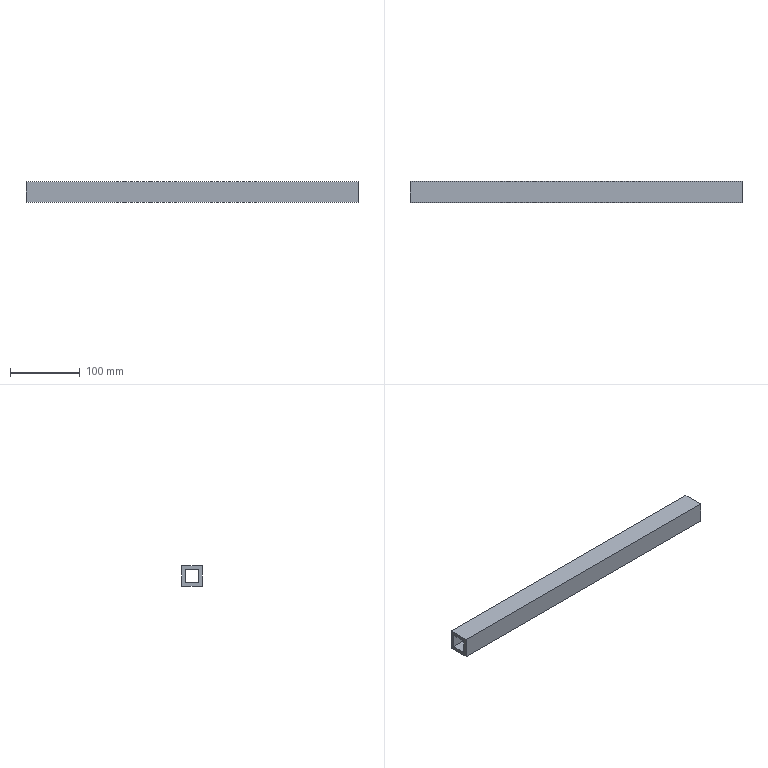Part | NX | features solid 2 | 1 solid | 10 faces | box 475 x 30 x 30 mm | volume 237500 mm3 | plane 10
STEP:
#1=CARTESIAN_POINT('',(650.,-165.,-80.));
#2=VERTEX_POINT('',#1);
#3=CARTESIAN_POINT('',(650.,-195.,-80.));
#4=VERTEX_POINT('',#3);
#5=CARTESIAN_POINT('',(650.,-165.,-80.));
#6=DIRECTION('',(0.,-1.,0.));
#7=VECTOR('',#6,1000.);
#8=LINE('',#5,#7);
#9=EDGE_CURVE('',#2,#4,#8,.T.);
#10=ORIENTED_EDGE('',*,*,#9,.F.);
#11=CARTESIAN_POINT('',(650.,-165.,-50.));
#12=VERTEX_POINT('',#11);
#13=CARTESIAN_POINT('',(650.,-165.,-50.));
#14=DIRECTION('',(0.,0.,-1.));
#15=VECTOR('',#14,1000.);
#16=LINE('',#13,#15);
#17=EDGE_CURVE('',#12,#2,#16,.T.);
#18=ORIENTED_EDGE('',*,*,#17,.F.);
#19=CARTESIAN_POINT('',(650.,-195.,-50.));
#20=VERTEX_POINT('',#19);
#21=CARTESIAN_POINT('',(650.,-165.,-50.));
#22=DIRECTION('',(0.,1.,0.));
#23=VECTOR('',#22,1000.);
#24=LINE('',#21,#23);
#25=EDGE_CURVE('',#12,#20,#24,.F.);
#26=ORIENTED_EDGE('',*,*,#25,.T.);
#27=CARTESIAN_POINT('',(650.,-195.,-50.));
#28=DIRECTION('',(0.,0.,1.));
#29=VECTOR('',#28,1000.);
#30=LINE('',#27,#29);
#31=EDGE_CURVE('',#20,#4,#30,.F.);
#32=ORIENTED_EDGE('',*,*,#31,.T.);
#33=EDGE_LOOP('',(#10,#18,#26,#32));
#34=FACE_BOUND('',#33,.T.);
#35=CARTESIAN_POINT('',(650.,-170.,-75.));
#36=VERTEX_POINT('',#35);
#37=CARTESIAN_POINT('',(650.,-190.,-75.));
#38=VERTEX_POINT('',#37);
#39=CARTESIAN_POINT('',(650.,-165.,-75.));
#40=DIRECTION('',(0.,-1.,0.));
#41=VECTOR('',#40,1000.);
#42=LINE('',#39,#41);
#43=EDGE_CURVE('',#36,#38,#42,.T.);
#44=ORIENTED_EDGE('',*,*,#43,.T.);
#45=CARTESIAN_POINT('',(650.,-190.,-55.));
#46=VERTEX_POINT('',#45);
#47=CARTESIAN_POINT('',(650.,-190.,-50.));
#48=DIRECTION('',(0.,0.,1.));
#49=VECTOR('',#48,1000.);
#50=LINE('',#47,#49);
#51=EDGE_CURVE('',#46,#38,#50,.F.);
#52=ORIENTED_EDGE('',*,*,#51,.F.);
#53=CARTESIAN_POINT('',(650.,-170.,-55.));
#54=VERTEX_POINT('',#53);
#55=CARTESIAN_POINT('',(650.,-165.,-55.));
#56=DIRECTION('',(0.,1.,0.));
#57=VECTOR('',#56,1000.);
#58=LINE('',#55,#57);
#59=EDGE_CURVE('',#54,#46,#58,.F.);
#60=ORIENTED_EDGE('',*,*,#59,.F.);
#61=CARTESIAN_POINT('',(650.,-170.,-50.));
#62=DIRECTION('',(0.,0.,-1.));
#63=VECTOR('',#62,1000.);
#64=LINE('',#61,#63);
#65=EDGE_CURVE('',#54,#36,#64,.T.);
#66=ORIENTED_EDGE('',*,*,#65,.T.);
#67=EDGE_LOOP('',(#44,#52,#60,#66));
#68=FACE_BOUND('',#67,.T.);
#69=CARTESIAN_POINT('',(650.,-165.,-50.));
#70=DIRECTION('',(-1.,0.,0.));
#71=DIRECTION('',(0.,0.,-1.));
#72=AXIS2_PLACEMENT_3D('',#69,#70,#71);
#73=PLANE('',#72);
#74=ADVANCED_FACE('',(#34,#68),#73,.F.);
#75=CARTESIAN_POINT('',(175.,-195.,-50.));
#76=VERTEX_POINT('',#75);
#77=CARTESIAN_POINT('',(140.,-195.,-50.));
#78=DIRECTION('',(1.,0.,0.));
#79=VECTOR('',#78,1000.);
#80=LINE('',#77,#79);
#81=EDGE_CURVE('',#20,#76,#80,.F.);
#82=ORIENTED_EDGE('',*,*,#81,.F.);
#83=ORIENTED_EDGE('',*,*,#25,.F.);
#84=CARTESIAN_POINT('',(175.,-165.,-50.));
#85=VERTEX_POINT('',#84);
#86=CARTESIAN_POINT('',(140.,-165.,-50.));
#87=DIRECTION('',(1.,0.,0.));
#88=VECTOR('',#87,1000.);
#89=LINE('',#86,#88);
#90=EDGE_CURVE('',#12,#85,#89,.F.);
#91=ORIENTED_EDGE('',*,*,#90,.T.);
#92=CARTESIAN_POINT('',(175.,20.,-50.));
#93=DIRECTION('',(0.,-1.,0.));
#94=VECTOR('',#93,1000.);
#95=LINE('',#92,#94);
#96=EDGE_CURVE('',#76,#85,#95,.F.);
#97=ORIENTED_EDGE('',*,*,#96,.F.);
#98=EDGE_LOOP('',(#82,#83,#91,#97));
#99=FACE_BOUND('',#98,.T.);
#100=CARTESIAN_POINT('',(140.,-165.,-50.));
#101=DIRECTION('',(0.,0.,1.));
#102=DIRECTION('',(0.,-1.,0.));
#103=AXIS2_PLACEMENT_3D('',#100,#101,#102);
#104=PLANE('',#103);
#105=ADVANCED_FACE('',(#99),#104,.T.);
#106=CARTESIAN_POINT('',(175.,-165.,-80.));
#107=VERTEX_POINT('',#106);
#108=CARTESIAN_POINT('',(140.,-165.,-80.));
#109=DIRECTION('',(1.,0.,0.));
#110=VECTOR('',#109,1000.);
#111=LINE('',#108,#110);
#112=EDGE_CURVE('',#2,#107,#111,.F.);
#113=ORIENTED_EDGE('',*,*,#112,.F.);
#114=ORIENTED_EDGE('',*,*,#9,.T.);
#115=CARTESIAN_POINT('',(175.,-195.,-80.));
#116=VERTEX_POINT('',#115);
#117=CARTESIAN_POINT('',(140.,-195.,-80.));
#118=DIRECTION('',(1.,0.,0.));
#119=VECTOR('',#118,1000.);
#120=LINE('',#117,#119);
#121=EDGE_CURVE('',#4,#116,#120,.F.);
#122=ORIENTED_EDGE('',*,*,#121,.T.);
#123=CARTESIAN_POINT('',(175.,20.,-80.));
#124=DIRECTION('',(0.,-1.,0.));
#125=VECTOR('',#124,1000.);
#126=LINE('',#123,#125);
#127=EDGE_CURVE('',#107,#116,#126,.T.);
#128=ORIENTED_EDGE('',*,*,#127,.F.);
#129=EDGE_LOOP('',(#113,#114,#122,#128));
#130=FACE_BOUND('',#129,.T.);
#131=CARTESIAN_POINT('',(140.,-165.,-80.));
#132=DIRECTION('',(0.,0.,1.));
#133=DIRECTION('',(0.,-1.,0.));
#134=AXIS2_PLACEMENT_3D('',#131,#132,#133);
#135=PLANE('',#134);
#136=ADVANCED_FACE('',(#130),#135,.F.);
#137=ORIENTED_EDGE('',*,*,#90,.F.);
#138=ORIENTED_EDGE('',*,*,#17,.T.);
#139=ORIENTED_EDGE('',*,*,#112,.T.);
#140=CARTESIAN_POINT('',(175.,-165.,-50.));
#141=DIRECTION('',(0.,0.,-1.));
#142=VECTOR('',#141,1000.);
#143=LINE('',#140,#142);
#144=EDGE_CURVE('',#85,#107,#143,.T.);
#145=ORIENTED_EDGE('',*,*,#144,.F.);
#146=EDGE_LOOP('',(#137,#138,#139,#145));
#147=FACE_BOUND('',#146,.T.);
#148=CARTESIAN_POINT('',(140.,-165.,-50.));
#149=DIRECTION('',(0.,-1.,0.));
#150=DIRECTION('',(0.,0.,-1.));
#151=AXIS2_PLACEMENT_3D('',#148,#149,#150);
#152=PLANE('',#151);
#153=ADVANCED_FACE('',(#147),#152,.F.);
#154=ORIENTED_EDGE('',*,*,#121,.F.);
#155=ORIENTED_EDGE('',*,*,#31,.F.);
#156=ORIENTED_EDGE('',*,*,#81,.T.);
#157=CARTESIAN_POINT('',(175.,-195.,-50.));
#158=DIRECTION('',(0.,0.,-1.));
#159=VECTOR('',#158,1000.);
#160=LINE('',#157,#159);
#161=EDGE_CURVE('',#116,#76,#160,.F.);
#162=ORIENTED_EDGE('',*,*,#161,.F.);
#163=EDGE_LOOP('',(#154,#155,#156,#162));
#164=FACE_BOUND('',#163,.T.);
#165=CARTESIAN_POINT('',(140.,-195.,-50.));
#166=DIRECTION('',(0.,-1.,0.));
#167=DIRECTION('',(0.,0.,-1.));
#168=AXIS2_PLACEMENT_3D('',#165,#166,#167);
#169=PLANE('',#168);
#170=ADVANCED_FACE('',(#164),#169,.T.);
#171=CARTESIAN_POINT('',(175.,-190.,-55.));
#172=VERTEX_POINT('',#171);
#173=CARTESIAN_POINT('',(175.,-170.,-55.));
#174=VERTEX_POINT('',#173);
#175=CARTESIAN_POINT('',(175.,20.,-55.));
#176=DIRECTION('',(0.,-1.,0.));
#177=VECTOR('',#176,1000.);
#178=LINE('',#175,#177);
#179=EDGE_CURVE('',#172,#174,#178,.F.);
#180=ORIENTED_EDGE('',*,*,#179,.T.);
#181=CARTESIAN_POINT('',(140.,-170.,-55.));
#182=DIRECTION('',(1.,0.,0.));
#183=VECTOR('',#182,1000.);
#184=LINE('',#181,#183);
#185=EDGE_CURVE('',#54,#174,#184,.F.);
#186=ORIENTED_EDGE('',*,*,#185,.F.);
#187=ORIENTED_EDGE('',*,*,#59,.T.);
#188=CARTESIAN_POINT('',(140.,-190.,-55.));
#189=DIRECTION('',(-1.,0.,0.));
#190=VECTOR('',#189,1000.);
#191=LINE('',#188,#190);
#192=EDGE_CURVE('',#46,#172,#191,.T.);
#193=ORIENTED_EDGE('',*,*,#192,.T.);
#194=EDGE_LOOP('',(#180,#186,#187,#193));
#195=FACE_BOUND('',#194,.T.);
#196=CARTESIAN_POINT('',(140.,-165.,-55.));
#197=DIRECTION('',(0.,0.,1.));
#198=DIRECTION('',(0.,-1.,0.));
#199=AXIS2_PLACEMENT_3D('',#196,#197,#198);
#200=PLANE('',#199);
#201=ADVANCED_FACE('',(#195),#200,.F.);
#202=CARTESIAN_POINT('',(175.,-170.,-75.));
#203=VERTEX_POINT('',#202);
#204=CARTESIAN_POINT('',(175.,-190.,-75.));
#205=VERTEX_POINT('',#204);
#206=CARTESIAN_POINT('',(175.,20.,-75.));
#207=DIRECTION('',(0.,-1.,0.));
#208=VECTOR('',#207,1000.);
#209=LINE('',#206,#208);
#210=EDGE_CURVE('',#203,#205,#209,.T.);
#211=ORIENTED_EDGE('',*,*,#210,.T.);
#212=CARTESIAN_POINT('',(140.,-190.,-75.));
#213=DIRECTION('',(1.,0.,0.));
#214=VECTOR('',#213,1000.);
#215=LINE('',#212,#214);
#216=EDGE_CURVE('',#38,#205,#215,.F.);
#217=ORIENTED_EDGE('',*,*,#216,.F.);
#218=ORIENTED_EDGE('',*,*,#43,.F.);
#219=CARTESIAN_POINT('',(140.,-170.,-75.));
#220=DIRECTION('',(-1.,0.,0.));
#221=VECTOR('',#220,1000.);
#222=LINE('',#219,#221);
#223=EDGE_CURVE('',#36,#203,#222,.T.);
#224=ORIENTED_EDGE('',*,*,#223,.T.);
#225=EDGE_LOOP('',(#211,#217,#218,#224));
#226=FACE_BOUND('',#225,.T.);
#227=CARTESIAN_POINT('',(140.,-165.,-75.));
#228=DIRECTION('',(0.,0.,1.));
#229=DIRECTION('',(0.,-1.,0.));
#230=AXIS2_PLACEMENT_3D('',#227,#228,#229);
#231=PLANE('',#230);
#232=ADVANCED_FACE('',(#226),#231,.T.);
#233=CARTESIAN_POINT('',(175.,-170.,-50.));
#234=DIRECTION('',(0.,0.,-1.));
#235=VECTOR('',#234,1000.);
#236=LINE('',#233,#235);
#237=EDGE_CURVE('',#174,#203,#236,.T.);
#238=ORIENTED_EDGE('',*,*,#237,.T.);
#239=ORIENTED_EDGE('',*,*,#223,.F.);
#240=ORIENTED_EDGE('',*,*,#65,.F.);
#241=ORIENTED_EDGE('',*,*,#185,.T.);
#242=EDGE_LOOP('',(#238,#239,#240,#241));
#243=FACE_BOUND('',#242,.T.);
#244=CARTESIAN_POINT('',(140.,-170.,-50.));
#245=DIRECTION('',(0.,-1.,0.));
#246=DIRECTION('',(0.,0.,-1.));
#247=AXIS2_PLACEMENT_3D('',#244,#245,#246);
#248=PLANE('',#247);
#249=ADVANCED_FACE('',(#243),#248,.T.);
#250=CARTESIAN_POINT('',(175.,-190.,-50.));
#251=DIRECTION('',(0.,0.,-1.));
#252=VECTOR('',#251,1000.);
#253=LINE('',#250,#252);
#254=EDGE_CURVE('',#205,#172,#253,.F.);
#255=ORIENTED_EDGE('',*,*,#254,.T.);
#256=ORIENTED_EDGE('',*,*,#192,.F.);
#257=ORIENTED_EDGE('',*,*,#51,.T.);
#258=ORIENTED_EDGE('',*,*,#216,.T.);
#259=EDGE_LOOP('',(#255,#256,#257,#258));
#260=FACE_BOUND('',#259,.T.);
#261=CARTESIAN_POINT('',(140.,-190.,-50.));
#262=DIRECTION('',(0.,-1.,0.));
#263=DIRECTION('',(0.,0.,-1.));
#264=AXIS2_PLACEMENT_3D('',#261,#262,#263);
#265=PLANE('',#264);
#266=ADVANCED_FACE('',(#260),#265,.F.);
#267=ORIENTED_EDGE('',*,*,#237,.F.);
#268=ORIENTED_EDGE('',*,*,#179,.F.);
#269=ORIENTED_EDGE('',*,*,#254,.F.);
#270=ORIENTED_EDGE('',*,*,#210,.F.);
#271=EDGE_LOOP('',(#267,#268,#269,#270));
#272=FACE_BOUND('',#271,.T.);
#273=ORIENTED_EDGE('',*,*,#96,.T.);
#274=ORIENTED_EDGE('',*,*,#144,.T.);
#275=ORIENTED_EDGE('',*,*,#127,.T.);
#276=ORIENTED_EDGE('',*,*,#161,.T.);
#277=EDGE_LOOP('',(#273,#274,#275,#276));
#278=FACE_BOUND('',#277,.T.);
#279=CARTESIAN_POINT('',(175.,20.,-50.));
#280=DIRECTION('',(1.,0.,0.));
#281=DIRECTION('',(0.,0.,1.));
#282=AXIS2_PLACEMENT_3D('',#279,#280,#281);
#283=PLANE('',#282);
#284=ADVANCED_FACE('',(#272,#278),#283,.F.);
#285=CLOSED_SHELL('',(#74,#105,#136,#153,#170,#201,#232,#249,#266,#284));
#286=MANIFOLD_SOLID_BREP('',#285);
#287=(LENGTH_UNIT()NAMED_UNIT(*)SI_UNIT(.MILLI.,.METRE.));
#288=UNCERTAINTY_MEASURE_WITH_UNIT(LENGTH_MEASURE(0.00001),#287,'','');
#289=(NAMED_UNIT(*)PLANE_ANGLE_UNIT()SI_UNIT($,.RADIAN.));
#290=(NAMED_UNIT(*)SI_UNIT($,.STERADIAN.)SOLID_ANGLE_UNIT());
#291=(GEOMETRIC_REPRESENTATION_CONTEXT(3)GLOBAL_UNCERTAINTY_ASSIGNED_CONTEXT((#288))GLOBAL_UNIT_ASSIGNED_CONTEXT((#287,#289,#290))REPRESENTATION_CONTEXT('',''));
#292=ADVANCED_BREP_SHAPE_REPRESENTATION('',(#286),#291);